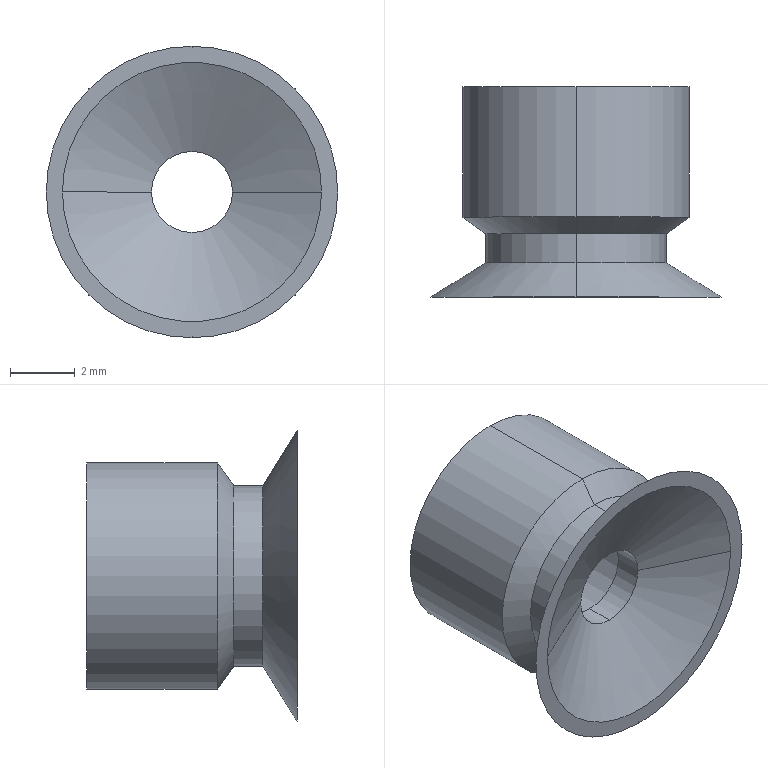Part | STEP file | PN_0033 | 1 solid | 18 faces | box 9 x 6.5 x 9 mm | volume 149.71 mm3 | cylinder 8 | cone 8 | plane 2 | commonest cylinder face diameters 2.5 x2 4.028 x2 5.56 x2 7 x2
STEP:
#1=CARTESIAN_POINT('',(0.,0.,0.));
#2=DIRECTION('',(0.,0.,1.));
#3=DIRECTION('',(1.,0.,0.));
#4=AXIS2_PLACEMENT_3D('',#1,#2,#3);
#5=CARTESIAN_POINT('',(0.,0.,-3.5));
#6=VERTEX_POINT('',#5);
#7=CARTESIAN_POINT('',(0.,0.,3.5));
#8=VERTEX_POINT('',#7);
#9=CARTESIAN_POINT('',(0.,0.,0.));
#10=DIRECTION('',(0.,-1.,0.));
#11=DIRECTION('',(0.,0.,-1.));
#12=AXIS2_PLACEMENT_3D('',#9,#10,#11);
#13=CIRCLE('',#12,3.5);
#14=CARTESIAN_POINT('',(0.,43.5,0.));
#15=DIRECTION('',(0.,-1.,0.));
#16=DIRECTION('',(0.,0.,-1.));
#17=AXIS2_PLACEMENT_3D('',#14,#15,#16);
#18=CYLINDRICAL_SURFACE('',#17,3.5);
#19=CARTESIAN_POINT('',(0.,43.5));
#20=DIRECTION('',(1.,0.));
#21=VECTOR('',#20,1.);
#22=LINE('',#19,#21);
#23=(GEOMETRIC_REPRESENTATION_CONTEXT(2)PARAMETRIC_REPRESENTATION_CONTEXT()REPRESENTATION_CONTEXT('',''));
#24=DEFINITIONAL_REPRESENTATION('',(#22),#23);
#25=PCURVE('',#18,#24);
#26=CARTESIAN_POINT('',(0.,0.,2.014));
#27=DIRECTION('',(0.,1.,0.));
#28=DIRECTION('',(0.,0.,1.));
#29=AXIS2_PLACEMENT_3D('',#26,#27,#28);
#30=PLANE('',#29);
#31=CARTESIAN_POINT('',(-5.514,0.));
#32=CARTESIAN_POINT('',(-5.514,6.062));
#33=CARTESIAN_POINT('',(-0.264,3.031));
#34=CARTESIAN_POINT('',(4.986,0.));
#35=CARTESIAN_POINT('',(-0.264,-3.031));
#36=CARTESIAN_POINT('',(-5.514,-6.062));
#37=CARTESIAN_POINT('',(-5.514,0.));
#38=(BOUNDED_CURVE()B_SPLINE_CURVE(2,(#31,#32,#33,#34,#35,#36,#37),.UNSPECIFIED.,.T.,.F.)B_SPLINE_CURVE_WITH_KNOTS((1,2,2,2,2,1),(-2.094,0.,2.094,4.189,6.283,8.378),.UNSPECIFIED.)CURVE()GEOMETRIC_REPRESENTATION_ITEM()RATIONAL_B_SPLINE_CURVE((1.,0.5,1.,0.5,1.,0.5,1.))REPRESENTATION_ITEM(''));
#39=(GEOMETRIC_REPRESENTATION_CONTEXT(2)PARAMETRIC_REPRESENTATION_CONTEXT()REPRESENTATION_CONTEXT('',''));
#40=DEFINITIONAL_REPRESENTATION('',(#38),#39);
#41=PCURVE('',#30,#40);
#42=SURFACE_CURVE('',#13,(#25,#41),.PCURVE_S1.);
#43=EDGE_CURVE('',#6,#8,#42,.T.);
#44=ORIENTED_EDGE('',*,*,#43,.T.);
#45=CARTESIAN_POINT('',(0.,-4.027,3.5));
#46=VERTEX_POINT('',#45);
#47=CARTESIAN_POINT('',(0.,43.5,3.5));
#48=DIRECTION('',(0.,-1.,0.));
#49=VECTOR('',#48,1.);
#50=LINE('',#47,#49);
#51=CARTESIAN_POINT('',(3.142,0.));
#52=DIRECTION('',(0.,1.));
#53=VECTOR('',#52,1.);
#54=LINE('',#51,#53);
#55=(GEOMETRIC_REPRESENTATION_CONTEXT(2)PARAMETRIC_REPRESENTATION_CONTEXT()REPRESENTATION_CONTEXT('',''));
#56=DEFINITIONAL_REPRESENTATION('',(#54),#55);
#57=PCURVE('',#18,#56);
#58=CARTESIAN_POINT('',(0.,43.5,0.));
#59=DIRECTION('',(0.,-1.,0.));
#60=DIRECTION('',(0.,0.,-1.));
#61=AXIS2_PLACEMENT_3D('',#58,#59,#60);
#62=CYLINDRICAL_SURFACE('',#61,3.5);
#63=CARTESIAN_POINT('',(3.142,0.));
#64=DIRECTION('',(0.,1.));
#65=VECTOR('',#64,1.);
#66=LINE('',#63,#65);
#67=(GEOMETRIC_REPRESENTATION_CONTEXT(2)PARAMETRIC_REPRESENTATION_CONTEXT()REPRESENTATION_CONTEXT('',''));
#68=DEFINITIONAL_REPRESENTATION('',(#66),#67);
#69=PCURVE('',#62,#68);
#70=SURFACE_CURVE('',#50,(#57,#69),.PCURVE_S1.);
#71=EDGE_CURVE('',#8,#46,#70,.T.);
#72=ORIENTED_EDGE('',*,*,#71,.T.);
#73=CARTESIAN_POINT('',(0.,-4.027,-3.5));
#74=VERTEX_POINT('',#73);
#75=CARTESIAN_POINT('',(0.,-4.027,0.));
#76=DIRECTION('',(0.,1.,0.));
#77=DIRECTION('',(0.,0.,-1.));
#78=AXIS2_PLACEMENT_3D('',#75,#76,#77);
#79=CIRCLE('',#78,3.5);
#80=CARTESIAN_POINT('',(6.283,47.527));
#81=DIRECTION('',(-1.,0.));
#82=VECTOR('',#81,1.);
#83=LINE('',#80,#82);
#84=(GEOMETRIC_REPRESENTATION_CONTEXT(2)PARAMETRIC_REPRESENTATION_CONTEXT()REPRESENTATION_CONTEXT('',''));
#85=DEFINITIONAL_REPRESENTATION('',(#83),#84);
#86=PCURVE('',#18,#85);
#87=CARTESIAN_POINT('',(0.,-4.027,0.));
#88=DIRECTION('',(0.,1.,0.));
#89=DIRECTION('',(0.,0.,1.));
#90=AXIS2_PLACEMENT_3D('',#87,#88,#89);
#91=CONICAL_SURFACE('',#90,3.5,0.9499);
#92=CARTESIAN_POINT('',(-3.142,0.));
#93=DIRECTION('',(1.,0.));
#94=VECTOR('',#93,1.);
#95=LINE('',#92,#94);
#96=(GEOMETRIC_REPRESENTATION_CONTEXT(2)PARAMETRIC_REPRESENTATION_CONTEXT()REPRESENTATION_CONTEXT('',''));
#97=DEFINITIONAL_REPRESENTATION('',(#95),#96);
#98=PCURVE('',#91,#97);
#99=SURFACE_CURVE('',#79,(#86,#98),.PCURVE_S1.);
#100=EDGE_CURVE('',#46,#74,#99,.T.);
#101=ORIENTED_EDGE('',*,*,#100,.T.);
#102=CARTESIAN_POINT('',(0.,43.5,-3.5));
#103=DIRECTION('',(0.,-1.,0.));
#104=VECTOR('',#103,1.);
#105=LINE('',#102,#104);
#106=CARTESIAN_POINT('',(0.,0.));
#107=DIRECTION('',(0.,1.));
#108=VECTOR('',#107,1.);
#109=LINE('',#106,#108);
#110=(GEOMETRIC_REPRESENTATION_CONTEXT(2)PARAMETRIC_REPRESENTATION_CONTEXT()REPRESENTATION_CONTEXT('',''));
#111=DEFINITIONAL_REPRESENTATION('',(#109),#110);
#112=PCURVE('',#18,#111);
#113=CARTESIAN_POINT('',(6.283,0.));
#114=DIRECTION('',(0.,1.));
#115=VECTOR('',#114,1.);
#116=LINE('',#113,#115);
#117=(GEOMETRIC_REPRESENTATION_CONTEXT(2)PARAMETRIC_REPRESENTATION_CONTEXT()REPRESENTATION_CONTEXT('',''));
#118=DEFINITIONAL_REPRESENTATION('',(#116),#117);
#119=PCURVE('',#62,#118);
#120=SURFACE_CURVE('',#105,(#112,#119),.PCURVE_S1.);
#121=EDGE_CURVE('',#6,#74,#120,.T.);
#122=ORIENTED_EDGE('',*,*,#121,.F.);
#123=EDGE_LOOP('',(#44,#72,#101,#122));
#124=FACE_BOUND('',#123,.T.);
#125=ADVANCED_FACE('',(#124),#18,.T.);
#126=CARTESIAN_POINT('',(0.,-4.542,2.78));
#127=VERTEX_POINT('',#126);
#128=CARTESIAN_POINT('',(0.,-4.542,-2.78));
#129=VERTEX_POINT('',#128);
#130=CARTESIAN_POINT('',(0.,-4.542,0.));
#131=DIRECTION('',(0.,1.,0.));
#132=DIRECTION('',(0.,0.,1.));
#133=AXIS2_PLACEMENT_3D('',#130,#131,#132);
#134=CIRCLE('',#133,2.78);
#135=CARTESIAN_POINT('',(0.,-0.515));
#136=DIRECTION('',(1.,0.));
#137=VECTOR('',#136,1.);
#138=LINE('',#135,#137);
#139=(GEOMETRIC_REPRESENTATION_CONTEXT(2)PARAMETRIC_REPRESENTATION_CONTEXT()REPRESENTATION_CONTEXT('',''));
#140=DEFINITIONAL_REPRESENTATION('',(#138),#139);
#141=PCURVE('',#91,#140);
#142=CARTESIAN_POINT('',(0.,43.5,0.));
#143=DIRECTION('',(0.,-1.,0.));
#144=DIRECTION('',(0.,0.,-1.));
#145=AXIS2_PLACEMENT_3D('',#142,#143,#144);
#146=CYLINDRICAL_SURFACE('',#145,2.78);
#147=CARTESIAN_POINT('',(3.142,48.042));
#148=DIRECTION('',(-1.,0.));
#149=VECTOR('',#148,1.);
#150=LINE('',#147,#149);
#151=(GEOMETRIC_REPRESENTATION_CONTEXT(2)PARAMETRIC_REPRESENTATION_CONTEXT()REPRESENTATION_CONTEXT('',''));
#152=DEFINITIONAL_REPRESENTATION('',(#150),#151);
#153=PCURVE('',#146,#152);
#154=SURFACE_CURVE('',#134,(#141,#153),.PCURVE_S1.);
#155=EDGE_CURVE('',#127,#129,#154,.T.);
#156=ORIENTED_EDGE('',*,*,#155,.T.);
#157=CARTESIAN_POINT('',(0.,-4.027,-3.5));
#158=DIRECTION('',(0.,0.5818,-0.8134));
#159=VECTOR('',#158,1.);
#160=LINE('',#157,#159);
#161=CARTESIAN_POINT('',(3.142,0.));
#162=DIRECTION('',(0.,1.));
#163=VECTOR('',#162,1.);
#164=LINE('',#161,#163);
#165=(GEOMETRIC_REPRESENTATION_CONTEXT(2)PARAMETRIC_REPRESENTATION_CONTEXT()REPRESENTATION_CONTEXT('',''));
#166=DEFINITIONAL_REPRESENTATION('',(#164),#165);
#167=PCURVE('',#91,#166);
#168=CARTESIAN_POINT('',(0.,-4.027,0.));
#169=DIRECTION('',(0.,1.,0.));
#170=DIRECTION('',(0.,0.,1.));
#171=AXIS2_PLACEMENT_3D('',#168,#169,#170);
#172=CONICAL_SURFACE('',#171,3.5,0.9499);
#173=CARTESIAN_POINT('',(3.142,0.));
#174=DIRECTION('',(0.,1.));
#175=VECTOR('',#174,1.);
#176=LINE('',#173,#175);
#177=(GEOMETRIC_REPRESENTATION_CONTEXT(2)PARAMETRIC_REPRESENTATION_CONTEXT()REPRESENTATION_CONTEXT('',''));
#178=DEFINITIONAL_REPRESENTATION('',(#176),#177);
#179=PCURVE('',#172,#178);
#180=SURFACE_CURVE('',#160,(#167,#179),.PCURVE_S1.);
#181=EDGE_CURVE('',#129,#74,#180,.T.);
#182=ORIENTED_EDGE('',*,*,#181,.T.);
#183=ORIENTED_EDGE('',*,*,#100,.F.);
#184=CARTESIAN_POINT('',(0.,-4.027,3.5));
#185=DIRECTION('',(0.,0.5818,0.8134));
#186=VECTOR('',#185,1.);
#187=LINE('',#184,#186);
#188=CARTESIAN_POINT('',(0.,0.));
#189=DIRECTION('',(0.,1.));
#190=VECTOR('',#189,1.);
#191=LINE('',#188,#190);
#192=(GEOMETRIC_REPRESENTATION_CONTEXT(2)PARAMETRIC_REPRESENTATION_CONTEXT()REPRESENTATION_CONTEXT('',''));
#193=DEFINITIONAL_REPRESENTATION('',(#191),#192);
#194=PCURVE('',#91,#193);
#195=CARTESIAN_POINT('',(6.283,0.));
#196=DIRECTION('',(0.,1.));
#197=VECTOR('',#196,1.);
#198=LINE('',#195,#197);
#199=(GEOMETRIC_REPRESENTATION_CONTEXT(2)PARAMETRIC_REPRESENTATION_CONTEXT()REPRESENTATION_CONTEXT('',''));
#200=DEFINITIONAL_REPRESENTATION('',(#198),#199);
#201=PCURVE('',#172,#200);
#202=SURFACE_CURVE('',#187,(#194,#201),.PCURVE_S1.);
#203=EDGE_CURVE('',#127,#46,#202,.T.);
#204=ORIENTED_EDGE('',*,*,#203,.F.);
#205=EDGE_LOOP('',(#156,#182,#183,#204));
#206=FACE_BOUND('',#205,.T.);
#207=ADVANCED_FACE('',(#206),#91,.T.);
#208=CARTESIAN_POINT('',(0.,0.,-2.014));
#209=VERTEX_POINT('',#208);
#210=CARTESIAN_POINT('',(0.,-3.84,-2.014));
#211=VERTEX_POINT('',#210);
#212=CARTESIAN_POINT('',(0.,43.5,-2.014));
#213=DIRECTION('',(0.,-1.,0.));
#214=VECTOR('',#213,1.);
#215=LINE('',#212,#214);
#216=CARTESIAN_POINT('',(0.,43.5,0.));
#217=DIRECTION('',(0.,-1.,0.));
#218=DIRECTION('',(0.,0.,-1.));
#219=AXIS2_PLACEMENT_3D('',#216,#217,#218);
#220=CYLINDRICAL_SURFACE('',#219,2.014);
#221=CARTESIAN_POINT('',(6.283,0.));
#222=DIRECTION('',(0.,1.));
#223=VECTOR('',#222,1.);
#224=LINE('',#221,#223);
#225=(GEOMETRIC_REPRESENTATION_CONTEXT(2)PARAMETRIC_REPRESENTATION_CONTEXT()REPRESENTATION_CONTEXT('',''));
#226=DEFINITIONAL_REPRESENTATION('',(#224),#225);
#227=PCURVE('',#220,#226);
#228=CARTESIAN_POINT('',(0.,43.5,0.));
#229=DIRECTION('',(0.,-1.,0.));
#230=DIRECTION('',(0.,0.,-1.));
#231=AXIS2_PLACEMENT_3D('',#228,#229,#230);
#232=CYLINDRICAL_SURFACE('',#231,2.014);
#233=CARTESIAN_POINT('',(0.,0.));
#234=DIRECTION('',(0.,1.));
#235=VECTOR('',#234,1.);
#236=LINE('',#233,#235);
#237=(GEOMETRIC_REPRESENTATION_CONTEXT(2)PARAMETRIC_REPRESENTATION_CONTEXT()REPRESENTATION_CONTEXT('',''));
#238=DEFINITIONAL_REPRESENTATION('',(#236),#237);
#239=PCURVE('',#232,#238);
#240=SURFACE_CURVE('',#215,(#227,#239),.PCURVE_S1.);
#241=EDGE_CURVE('',#209,#211,#240,.T.);
#242=ORIENTED_EDGE('',*,*,#241,.T.);
#243=CARTESIAN_POINT('',(-2.014,-3.84,0.));
#244=VERTEX_POINT('',#243);
#245=CARTESIAN_POINT('',(0.,-3.84,0.));
#246=DIRECTION('',(0.,1.,0.));
#247=DIRECTION('',(0.,0.,-1.));
#248=AXIS2_PLACEMENT_3D('',#245,#246,#247);
#249=CIRCLE('',#248,2.014);
#250=CARTESIAN_POINT('',(6.283,47.34));
#251=DIRECTION('',(-1.,0.));
#252=VECTOR('',#251,1.);
#253=LINE('',#250,#252);
#254=(GEOMETRIC_REPRESENTATION_CONTEXT(2)PARAMETRIC_REPRESENTATION_CONTEXT()REPRESENTATION_CONTEXT('',''));
#255=DEFINITIONAL_REPRESENTATION('',(#253),#254);
#256=PCURVE('',#220,#255);
#257=CARTESIAN_POINT('',(0.,-3.84,0.));
#258=DIRECTION('',(0.,1.,0.));
#259=DIRECTION('',(-1.,0.,0.));
#260=AXIS2_PLACEMENT_3D('',#257,#258,#259);
#261=CONICAL_SURFACE('',#260,2.014,0.9822);
#262=CARTESIAN_POINT('',(4.712,0.));
#263=DIRECTION('',(1.,0.));
#264=VECTOR('',#263,1.);
#265=LINE('',#262,#264);
#266=(GEOMETRIC_REPRESENTATION_CONTEXT(2)PARAMETRIC_REPRESENTATION_CONTEXT()REPRESENTATION_CONTEXT('',''));
#267=DEFINITIONAL_REPRESENTATION('',(#265),#266);
#268=PCURVE('',#261,#267);
#269=SURFACE_CURVE('',#249,(#256,#268),.PCURVE_S1.);
#270=EDGE_CURVE('',#211,#244,#269,.T.);
#271=ORIENTED_EDGE('',*,*,#270,.T.);
#272=CARTESIAN_POINT('',(0.,-3.84,2.014));
#273=VERTEX_POINT('',#272);
#274=CARTESIAN_POINT('',(0.,-3.84,0.));
#275=DIRECTION('',(0.,1.,0.));
#276=DIRECTION('',(0.,0.,-1.));
#277=AXIS2_PLACEMENT_3D('',#274,#275,#276);
#278=CIRCLE('',#277,2.014);
#279=CARTESIAN_POINT('',(6.283,47.34));
#280=DIRECTION('',(-1.,0.));
#281=VECTOR('',#280,1.);
#282=LINE('',#279,#281);
#283=(GEOMETRIC_REPRESENTATION_CONTEXT(2)PARAMETRIC_REPRESENTATION_CONTEXT()REPRESENTATION_CONTEXT('',''));
#284=DEFINITIONAL_REPRESENTATION('',(#282),#283);
#285=PCURVE('',#220,#284);
#286=CARTESIAN_POINT('',(0.,-3.84,0.));
#287=DIRECTION('',(0.,1.,0.));
#288=DIRECTION('',(-1.,0.,0.));
#289=AXIS2_PLACEMENT_3D('',#286,#287,#288);
#290=CONICAL_SURFACE('',#289,2.014,0.9822);
#291=CARTESIAN_POINT('',(-1.571,0.));
#292=DIRECTION('',(1.,0.));
#293=VECTOR('',#292,1.);
#294=LINE('',#291,#293);
#295=(GEOMETRIC_REPRESENTATION_CONTEXT(2)PARAMETRIC_REPRESENTATION_CONTEXT()REPRESENTATION_CONTEXT('',''));
#296=DEFINITIONAL_REPRESENTATION('',(#294),#295);
#297=PCURVE('',#290,#296);
#298=SURFACE_CURVE('',#278,(#285,#297),.PCURVE_S1.);
#299=EDGE_CURVE('',#244,#273,#298,.T.);
#300=ORIENTED_EDGE('',*,*,#299,.T.);
#301=CARTESIAN_POINT('',(0.,0.,2.014));
#302=VERTEX_POINT('',#301);
#303=CARTESIAN_POINT('',(0.,43.5,2.014));
#304=DIRECTION('',(0.,-1.,0.));
#305=VECTOR('',#304,1.);
#306=LINE('',#303,#305);
#307=CARTESIAN_POINT('',(3.142,0.));
#308=DIRECTION('',(0.,1.));
#309=VECTOR('',#308,1.);
#310=LINE('',#307,#309);
#311=(GEOMETRIC_REPRESENTATION_CONTEXT(2)PARAMETRIC_REPRESENTATION_CONTEXT()REPRESENTATION_CONTEXT('',''));
#312=DEFINITIONAL_REPRESENTATION('',(#310),#311);
#313=PCURVE('',#220,#312);
#314=CARTESIAN_POINT('',(3.142,0.));
#315=DIRECTION('',(0.,1.));
#316=VECTOR('',#315,1.);
#317=LINE('',#314,#316);
#318=(GEOMETRIC_REPRESENTATION_CONTEXT(2)PARAMETRIC_REPRESENTATION_CONTEXT()REPRESENTATION_CONTEXT('',''));
#319=DEFINITIONAL_REPRESENTATION('',(#317),#318);
#320=PCURVE('',#232,#319);
#321=SURFACE_CURVE('',#306,(#313,#320),.PCURVE_S1.);
#322=EDGE_CURVE('',#302,#273,#321,.T.);
#323=ORIENTED_EDGE('',*,*,#322,.F.);
#324=CARTESIAN_POINT('',(0.,0.,0.));
#325=DIRECTION('',(0.,-1.,0.));
#326=DIRECTION('',(0.,0.,-1.));
#327=AXIS2_PLACEMENT_3D('',#324,#325,#326);
#328=CIRCLE('',#327,2.014);
#329=CARTESIAN_POINT('',(0.,43.5));
#330=DIRECTION('',(1.,0.));
#331=VECTOR('',#330,1.);
#332=LINE('',#329,#331);
#333=(GEOMETRIC_REPRESENTATION_CONTEXT(2)PARAMETRIC_REPRESENTATION_CONTEXT()REPRESENTATION_CONTEXT('',''));
#334=DEFINITIONAL_REPRESENTATION('',(#332),#333);
#335=PCURVE('',#220,#334);
#336=CARTESIAN_POINT('',(-4.028,0.));
#337=CARTESIAN_POINT('',(-4.028,3.488));
#338=CARTESIAN_POINT('',(-1.007,1.744));
#339=CARTESIAN_POINT('',(2.014,0.));
#340=CARTESIAN_POINT('',(-1.007,-1.744));
#341=CARTESIAN_POINT('',(-4.028,-3.488));
#342=CARTESIAN_POINT('',(-4.028,0.));
#343=(BOUNDED_CURVE()B_SPLINE_CURVE(2,(#336,#337,#338,#339,#340,#341,#342),.UNSPECIFIED.,.T.,.F.)B_SPLINE_CURVE_WITH_KNOTS((1,2,2,2,2,1),(-2.094,0.,2.094,4.189,6.283,8.378),.UNSPECIFIED.)CURVE()GEOMETRIC_REPRESENTATION_ITEM()RATIONAL_B_SPLINE_CURVE((1.,0.5,1.,0.5,1.,0.5,1.))REPRESENTATION_ITEM(''));
#344=(GEOMETRIC_REPRESENTATION_CONTEXT(2)PARAMETRIC_REPRESENTATION_CONTEXT()REPRESENTATION_CONTEXT('',''));
#345=DEFINITIONAL_REPRESENTATION('',(#343),#344);
#346=PCURVE('',#30,#345);
#347=SURFACE_CURVE('',#328,(#335,#346),.PCURVE_S1.);
#348=EDGE_CURVE('',#302,#209,#347,.T.);
#349=ORIENTED_EDGE('',*,*,#348,.T.);
#350=EDGE_LOOP('',(#242,#271,#300,#323,#349));
#351=FACE_BOUND('',#350,.F.);
#352=ADVANCED_FACE('',(#351),#220,.F.);
#353=ORIENTED_EDGE('',*,*,#155,.F.);
#354=CARTESIAN_POINT('',(0.,-5.439,2.78));
#355=VERTEX_POINT('',#354);
#356=CARTESIAN_POINT('',(0.,43.5,2.78));
#357=DIRECTION('',(0.,-1.,0.));
#358=VECTOR('',#357,1.);
#359=LINE('',#356,#358);
#360=CARTESIAN_POINT('',(3.142,0.));
#361=DIRECTION('',(0.,1.));
#362=VECTOR('',#361,1.);
#363=LINE('',#360,#362);
#364=(GEOMETRIC_REPRESENTATION_CONTEXT(2)PARAMETRIC_REPRESENTATION_CONTEXT()REPRESENTATION_CONTEXT('',''));
#365=DEFINITIONAL_REPRESENTATION('',(#363),#364);
#366=PCURVE('',#146,#365);
#367=CARTESIAN_POINT('',(0.,43.5,0.));
#368=DIRECTION('',(0.,-1.,0.));
#369=DIRECTION('',(0.,0.,-1.));
#370=AXIS2_PLACEMENT_3D('',#367,#368,#369);
#371=CYLINDRICAL_SURFACE('',#370,2.78);
#372=CARTESIAN_POINT('',(3.142,0.));
#373=DIRECTION('',(0.,1.));
#374=VECTOR('',#373,1.);
#375=LINE('',#372,#374);
#376=(GEOMETRIC_REPRESENTATION_CONTEXT(2)PARAMETRIC_REPRESENTATION_CONTEXT()REPRESENTATION_CONTEXT('',''));
#377=DEFINITIONAL_REPRESENTATION('',(#375),#376);
#378=PCURVE('',#371,#377);
#379=SURFACE_CURVE('',#359,(#366,#378),.PCURVE_S1.);
#380=EDGE_CURVE('',#127,#355,#379,.T.);
#381=ORIENTED_EDGE('',*,*,#380,.T.);
#382=CARTESIAN_POINT('',(0.,-5.439,-2.78));
#383=VERTEX_POINT('',#382);
#384=CARTESIAN_POINT('',(0.,-5.439,0.));
#385=DIRECTION('',(0.,1.,0.));
#386=DIRECTION('',(0.,0.,-1.));
#387=AXIS2_PLACEMENT_3D('',#384,#385,#386);
#388=CIRCLE('',#387,2.78);
#389=CARTESIAN_POINT('',(6.283,48.939));
#390=DIRECTION('',(-1.,0.));
#391=VECTOR('',#390,1.);
#392=LINE('',#389,#391);
#393=(GEOMETRIC_REPRESENTATION_CONTEXT(2)PARAMETRIC_REPRESENTATION_CONTEXT()REPRESENTATION_CONTEXT('',''));
#394=DEFINITIONAL_REPRESENTATION('',(#392),#393);
#395=PCURVE('',#146,#394);
#396=CARTESIAN_POINT('',(0.,-6.5,0.));
#397=DIRECTION('',(0.,-1.,0.));
#398=DIRECTION('',(0.,0.,-1.));
#399=AXIS2_PLACEMENT_3D('',#396,#397,#398);
#400=CONICAL_SURFACE('',#399,4.5,1.018);
#401=CARTESIAN_POINT('',(6.283,-1.061));
#402=DIRECTION('',(-1.,0.));
#403=VECTOR('',#402,1.);
#404=LINE('',#401,#403);
#405=(GEOMETRIC_REPRESENTATION_CONTEXT(2)PARAMETRIC_REPRESENTATION_CONTEXT()REPRESENTATION_CONTEXT('',''));
#406=DEFINITIONAL_REPRESENTATION('',(#404),#405);
#407=PCURVE('',#400,#406);
#408=SURFACE_CURVE('',#388,(#395,#407),.PCURVE_S1.);
#409=EDGE_CURVE('',#355,#383,#408,.T.);
#410=ORIENTED_EDGE('',*,*,#409,.T.);
#411=CARTESIAN_POINT('',(0.,43.5,-2.78));
#412=DIRECTION('',(0.,-1.,0.));
#413=VECTOR('',#412,1.);
#414=LINE('',#411,#413);
#415=CARTESIAN_POINT('',(0.,0.));
#416=DIRECTION('',(0.,1.));
#417=VECTOR('',#416,1.);
#418=LINE('',#415,#417);
#419=(GEOMETRIC_REPRESENTATION_CONTEXT(2)PARAMETRIC_REPRESENTATION_CONTEXT()REPRESENTATION_CONTEXT('',''));
#420=DEFINITIONAL_REPRESENTATION('',(#418),#419);
#421=PCURVE('',#146,#420);
#422=CARTESIAN_POINT('',(6.283,0.));
#423=DIRECTION('',(0.,1.));
#424=VECTOR('',#423,1.);
#425=LINE('',#422,#424);
#426=(GEOMETRIC_REPRESENTATION_CONTEXT(2)PARAMETRIC_REPRESENTATION_CONTEXT()REPRESENTATION_CONTEXT('',''));
#427=DEFINITIONAL_REPRESENTATION('',(#425),#426);
#428=PCURVE('',#371,#427);
#429=SURFACE_CURVE('',#414,(#421,#428),.PCURVE_S1.);
#430=EDGE_CURVE('',#129,#383,#429,.T.);
#431=ORIENTED_EDGE('',*,*,#430,.F.);
#432=EDGE_LOOP('',(#353,#381,#410,#431));
#433=FACE_BOUND('',#432,.T.);
#434=ADVANCED_FACE('',(#433),#146,.T.);
#435=CARTESIAN_POINT('',(0.,-4.35,-1.25));
#436=VERTEX_POINT('',#435);
#437=CARTESIAN_POINT('',(-1.25,-4.35,0.));
#438=VERTEX_POINT('',#437);
#439=CARTESIAN_POINT('',(0.,-4.35,0.));
#440=DIRECTION('',(0.,1.,0.));
#441=DIRECTION('',(0.,0.,1.));
#442=AXIS2_PLACEMENT_3D('',#439,#440,#441);
#443=CIRCLE('',#442,1.25);
#444=CARTESIAN_POINT('',(1.571,-0.51));
#445=DIRECTION('',(1.,0.));
#446=VECTOR('',#445,1.);
#447=LINE('',#444,#446);
#448=(GEOMETRIC_REPRESENTATION_CONTEXT(2)PARAMETRIC_REPRESENTATION_CONTEXT()REPRESENTATION_CONTEXT('',''));
#449=DEFINITIONAL_REPRESENTATION('',(#447),#448);
#450=PCURVE('',#261,#449);
#451=CARTESIAN_POINT('',(0.,43.5,0.));
#452=DIRECTION('',(0.,-1.,0.));
#453=DIRECTION('',(0.,0.,-1.));
#454=AXIS2_PLACEMENT_3D('',#451,#452,#453);
#455=CYLINDRICAL_SURFACE('',#454,1.25);
#456=CARTESIAN_POINT('',(9.425,47.85));
#457=DIRECTION('',(-1.,0.));
#458=VECTOR('',#457,1.);
#459=LINE('',#456,#458);
#460=(GEOMETRIC_REPRESENTATION_CONTEXT(2)PARAMETRIC_REPRESENTATION_CONTEXT()REPRESENTATION_CONTEXT('',''));
#461=DEFINITIONAL_REPRESENTATION('',(#459),#460);
#462=PCURVE('',#455,#461);
#463=SURFACE_CURVE('',#443,(#450,#462),.PCURVE_S1.);
#464=EDGE_CURVE('',#436,#438,#463,.T.);
#465=ORIENTED_EDGE('',*,*,#464,.T.);
#466=CARTESIAN_POINT('',(-2.014,-3.84,0.));
#467=DIRECTION('',(-0.8317,0.5552,0.));
#468=VECTOR('',#467,1.);
#469=LINE('',#466,#468);
#470=CARTESIAN_POINT('',(6.283,0.));
#471=DIRECTION('',(0.,1.));
#472=VECTOR('',#471,1.);
#473=LINE('',#470,#472);
#474=(GEOMETRIC_REPRESENTATION_CONTEXT(2)PARAMETRIC_REPRESENTATION_CONTEXT()REPRESENTATION_CONTEXT('',''));
#475=DEFINITIONAL_REPRESENTATION('',(#473),#474);
#476=PCURVE('',#261,#475);
#477=CARTESIAN_POINT('',(0.,0.));
#478=DIRECTION('',(0.,1.));
#479=VECTOR('',#478,1.);
#480=LINE('',#477,#479);
#481=(GEOMETRIC_REPRESENTATION_CONTEXT(2)PARAMETRIC_REPRESENTATION_CONTEXT()REPRESENTATION_CONTEXT('',''));
#482=DEFINITIONAL_REPRESENTATION('',(#480),#481);
#483=PCURVE('',#290,#482);
#484=SURFACE_CURVE('',#469,(#476,#483),.PCURVE_S1.);
#485=EDGE_CURVE('',#438,#244,#484,.T.);
#486=ORIENTED_EDGE('',*,*,#485,.T.);
#487=ORIENTED_EDGE('',*,*,#270,.F.);
#488=CARTESIAN_POINT('',(2.014,-3.84,0.));
#489=VERTEX_POINT('',#488);
#490=CARTESIAN_POINT('',(0.,-3.84,0.));
#491=DIRECTION('',(0.,1.,0.));
#492=DIRECTION('',(0.,0.,-1.));
#493=AXIS2_PLACEMENT_3D('',#490,#491,#492);
#494=CIRCLE('',#493,2.014);
#495=CARTESIAN_POINT('',(-1.571,0.));
#496=DIRECTION('',(1.,0.));
#497=VECTOR('',#496,1.);
#498=LINE('',#495,#497);
#499=(GEOMETRIC_REPRESENTATION_CONTEXT(2)PARAMETRIC_REPRESENTATION_CONTEXT()REPRESENTATION_CONTEXT('',''));
#500=DEFINITIONAL_REPRESENTATION('',(#498),#499);
#501=PCURVE('',#261,#500);
#502=CARTESIAN_POINT('',(6.283,47.34));
#503=DIRECTION('',(-1.,0.));
#504=VECTOR('',#503,1.);
#505=LINE('',#502,#504);
#506=(GEOMETRIC_REPRESENTATION_CONTEXT(2)PARAMETRIC_REPRESENTATION_CONTEXT()REPRESENTATION_CONTEXT('',''));
#507=DEFINITIONAL_REPRESENTATION('',(#505),#506);
#508=PCURVE('',#232,#507);
#509=SURFACE_CURVE('',#494,(#501,#508),.PCURVE_S1.);
#510=EDGE_CURVE('',#489,#211,#509,.T.);
#511=ORIENTED_EDGE('',*,*,#510,.F.);
#512=CARTESIAN_POINT('',(1.25,-4.35,0.));
#513=VERTEX_POINT('',#512);
#514=CARTESIAN_POINT('',(2.014,-3.84,0.));
#515=DIRECTION('',(0.8317,0.5552,0.));
#516=VECTOR('',#515,1.);
#517=LINE('',#514,#516);
#518=CARTESIAN_POINT('',(3.142,0.));
#519=DIRECTION('',(0.,1.));
#520=VECTOR('',#519,1.);
#521=LINE('',#518,#520);
#522=(GEOMETRIC_REPRESENTATION_CONTEXT(2)PARAMETRIC_REPRESENTATION_CONTEXT()REPRESENTATION_CONTEXT('',''));
#523=DEFINITIONAL_REPRESENTATION('',(#521),#522);
#524=PCURVE('',#261,#523);
#525=CARTESIAN_POINT('',(3.142,0.));
#526=DIRECTION('',(0.,1.));
#527=VECTOR('',#526,1.);
#528=LINE('',#525,#527);
#529=(GEOMETRIC_REPRESENTATION_CONTEXT(2)PARAMETRIC_REPRESENTATION_CONTEXT()REPRESENTATION_CONTEXT('',''));
#530=DEFINITIONAL_REPRESENTATION('',(#528),#529);
#531=PCURVE('',#290,#530);
#532=SURFACE_CURVE('',#517,(#524,#531),.PCURVE_S1.);
#533=EDGE_CURVE('',#513,#489,#532,.T.);
#534=ORIENTED_EDGE('',*,*,#533,.F.);
#535=CARTESIAN_POINT('',(0.,-4.35,0.));
#536=DIRECTION('',(0.,1.,0.));
#537=DIRECTION('',(0.,0.,1.));
#538=AXIS2_PLACEMENT_3D('',#535,#536,#537);
#539=CIRCLE('',#538,1.25);
#540=CARTESIAN_POINT('',(1.571,-0.51));
#541=DIRECTION('',(1.,0.));
#542=VECTOR('',#541,1.);
#543=LINE('',#540,#542);
#544=(GEOMETRIC_REPRESENTATION_CONTEXT(2)PARAMETRIC_REPRESENTATION_CONTEXT()REPRESENTATION_CONTEXT('',''));
#545=DEFINITIONAL_REPRESENTATION('',(#543),#544);
#546=PCURVE('',#261,#545);
#547=CARTESIAN_POINT('',(0.,43.5,0.));
#548=DIRECTION('',(0.,-1.,0.));
#549=DIRECTION('',(0.,0.,-1.));
#550=AXIS2_PLACEMENT_3D('',#547,#548,#549);
#551=CYLINDRICAL_SURFACE('',#550,1.25);
#552=CARTESIAN_POINT('',(3.142,47.85));
#553=DIRECTION('',(-1.,0.));
#554=VECTOR('',#553,1.);
#555=LINE('',#552,#554);
#556=(GEOMETRIC_REPRESENTATION_CONTEXT(2)PARAMETRIC_REPRESENTATION_CONTEXT()REPRESENTATION_CONTEXT('',''));
#557=DEFINITIONAL_REPRESENTATION('',(#555),#556);
#558=PCURVE('',#551,#557);
#559=SURFACE_CURVE('',#539,(#546,#558),.PCURVE_S1.);
#560=EDGE_CURVE('',#513,#436,#559,.T.);
#561=ORIENTED_EDGE('',*,*,#560,.T.);
#562=EDGE_LOOP('',(#465,#486,#487,#511,#534,#561));
#563=FACE_BOUND('',#562,.F.);
#564=ADVANCED_FACE('',(#563),#261,.F.);
#565=ORIENTED_EDGE('',*,*,#409,.F.);
#566=CARTESIAN_POINT('',(0.,-6.5,4.5));
#567=VERTEX_POINT('',#566);
#568=CARTESIAN_POINT('',(0.,-6.5,4.5));
#569=DIRECTION('',(0.,-0.525,0.8511));
#570=VECTOR('',#569,1.);
#571=LINE('',#568,#570);
#572=CARTESIAN_POINT('',(3.142,0.));
#573=DIRECTION('',(0.,1.));
#574=VECTOR('',#573,1.);
#575=LINE('',#572,#574);
#576=(GEOMETRIC_REPRESENTATION_CONTEXT(2)PARAMETRIC_REPRESENTATION_CONTEXT()REPRESENTATION_CONTEXT('',''));
#577=DEFINITIONAL_REPRESENTATION('',(#575),#576);
#578=PCURVE('',#400,#577);
#579=CARTESIAN_POINT('',(0.,-6.5,0.));
#580=DIRECTION('',(0.,-1.,0.));
#581=DIRECTION('',(0.,0.,-1.));
#582=AXIS2_PLACEMENT_3D('',#579,#580,#581);
#583=CONICAL_SURFACE('',#582,4.5,1.018);
#584=CARTESIAN_POINT('',(3.142,0.));
#585=DIRECTION('',(0.,1.));
#586=VECTOR('',#585,1.);
#587=LINE('',#584,#586);
#588=(GEOMETRIC_REPRESENTATION_CONTEXT(2)PARAMETRIC_REPRESENTATION_CONTEXT()REPRESENTATION_CONTEXT('',''));
#589=DEFINITIONAL_REPRESENTATION('',(#587),#588);
#590=PCURVE('',#583,#589);
#591=SURFACE_CURVE('',#571,(#578,#590),.PCURVE_S1.);
#592=EDGE_CURVE('',#355,#567,#591,.T.);
#593=ORIENTED_EDGE('',*,*,#592,.T.);
#594=CARTESIAN_POINT('',(0.,-6.5,-4.5));
#595=VERTEX_POINT('',#594);
#596=CARTESIAN_POINT('',(0.,-6.5,0.));
#597=DIRECTION('',(0.,1.,0.));
#598=DIRECTION('',(0.,0.,-1.));
#599=AXIS2_PLACEMENT_3D('',#596,#597,#598);
#600=CIRCLE('',#599,4.5);
#601=CARTESIAN_POINT('',(6.283,0.));
#602=DIRECTION('',(-1.,0.));
#603=VECTOR('',#602,1.);
#604=LINE('',#601,#603);
#605=(GEOMETRIC_REPRESENTATION_CONTEXT(2)PARAMETRIC_REPRESENTATION_CONTEXT()REPRESENTATION_CONTEXT('',''));
#606=DEFINITIONAL_REPRESENTATION('',(#604),#605);
#607=PCURVE('',#400,#606);
#608=CARTESIAN_POINT('',(0.,-6.5,4.5));
#609=DIRECTION('',(0.,-1.,0.));
#610=DIRECTION('',(0.,0.,-1.));
#611=AXIS2_PLACEMENT_3D('',#608,#609,#610);
#612=PLANE('',#611);
#613=CARTESIAN_POINT('',(9.,0.));
#614=CARTESIAN_POINT('',(9.,-7.794));
#615=CARTESIAN_POINT('',(2.25,-3.897));
#616=CARTESIAN_POINT('',(-4.5,0.));
#617=CARTESIAN_POINT('',(2.25,3.897));
#618=CARTESIAN_POINT('',(9.,7.794));
#619=CARTESIAN_POINT('',(9.,0.));
#620=(BOUNDED_CURVE()B_SPLINE_CURVE(2,(#613,#614,#615,#616,#617,#618,#619),.UNSPECIFIED.,.T.,.F.)B_SPLINE_CURVE_WITH_KNOTS((1,2,2,2,2,1),(-2.094,0.,2.094,4.189,6.283,8.378),.UNSPECIFIED.)CURVE()GEOMETRIC_REPRESENTATION_ITEM()RATIONAL_B_SPLINE_CURVE((1.,0.5,1.,0.5,1.,0.5,1.))REPRESENTATION_ITEM(''));
#621=(GEOMETRIC_REPRESENTATION_CONTEXT(2)PARAMETRIC_REPRESENTATION_CONTEXT()REPRESENTATION_CONTEXT('',''));
#622=DEFINITIONAL_REPRESENTATION('',(#620),#621);
#623=PCURVE('',#612,#622);
#624=SURFACE_CURVE('',#600,(#607,#623),.PCURVE_S1.);
#625=EDGE_CURVE('',#567,#595,#624,.T.);
#626=ORIENTED_EDGE('',*,*,#625,.T.);
#627=CARTESIAN_POINT('',(0.,-6.5,-4.5));
#628=DIRECTION('',(0.,-0.525,-0.8511));
#629=VECTOR('',#628,1.);
#630=LINE('',#627,#629);
#631=CARTESIAN_POINT('',(0.,0.));
#632=DIRECTION('',(0.,1.));
#633=VECTOR('',#632,1.);
#634=LINE('',#631,#633);
#635=(GEOMETRIC_REPRESENTATION_CONTEXT(2)PARAMETRIC_REPRESENTATION_CONTEXT()REPRESENTATION_CONTEXT('',''));
#636=DEFINITIONAL_REPRESENTATION('',(#634),#635);
#637=PCURVE('',#400,#636);
#638=CARTESIAN_POINT('',(6.283,0.));
#639=DIRECTION('',(0.,1.));
#640=VECTOR('',#639,1.);
#641=LINE('',#638,#640);
#642=(GEOMETRIC_REPRESENTATION_CONTEXT(2)PARAMETRIC_REPRESENTATION_CONTEXT()REPRESENTATION_CONTEXT('',''));
#643=DEFINITIONAL_REPRESENTATION('',(#641),#642);
#644=PCURVE('',#583,#643);
#645=SURFACE_CURVE('',#630,(#637,#644),.PCURVE_S1.);
#646=EDGE_CURVE('',#383,#595,#645,.T.);
#647=ORIENTED_EDGE('',*,*,#646,.F.);
#648=EDGE_LOOP('',(#565,#593,#626,#647));
#649=FACE_BOUND('',#648,.T.);
#650=ADVANCED_FACE('',(#649),#400,.T.);
#651=CARTESIAN_POINT('',(0.,-5.206,-1.25));
#652=VERTEX_POINT('',#651);
#653=CARTESIAN_POINT('',(0.,43.5,-1.25));
#654=DIRECTION('',(0.,-1.,0.));
#655=VECTOR('',#654,1.);
#656=LINE('',#653,#655);
#657=CARTESIAN_POINT('',(6.283,0.));
#658=DIRECTION('',(0.,1.));
#659=VECTOR('',#658,1.);
#660=LINE('',#657,#659);
#661=(GEOMETRIC_REPRESENTATION_CONTEXT(2)PARAMETRIC_REPRESENTATION_CONTEXT()REPRESENTATION_CONTEXT('',''));
#662=DEFINITIONAL_REPRESENTATION('',(#660),#661);
#663=PCURVE('',#455,#662);
#664=CARTESIAN_POINT('',(0.,0.));
#665=DIRECTION('',(0.,1.));
#666=VECTOR('',#665,1.);
#667=LINE('',#664,#666);
#668=(GEOMETRIC_REPRESENTATION_CONTEXT(2)PARAMETRIC_REPRESENTATION_CONTEXT()REPRESENTATION_CONTEXT('',''));
#669=DEFINITIONAL_REPRESENTATION('',(#667),#668);
#670=PCURVE('',#551,#669);
#671=SURFACE_CURVE('',#656,(#663,#670),.PCURVE_S1.);
#672=EDGE_CURVE('',#436,#652,#671,.T.);
#673=ORIENTED_EDGE('',*,*,#672,.T.);
#674=CARTESIAN_POINT('',(-1.25,-5.206,0.));
#675=VERTEX_POINT('',#674);
#676=CARTESIAN_POINT('',(0.,-5.206,0.));
#677=DIRECTION('',(0.,1.,0.));
#678=DIRECTION('',(0.,0.,-1.));
#679=AXIS2_PLACEMENT_3D('',#676,#677,#678);
#680=CIRCLE('',#679,1.25);
#681=CARTESIAN_POINT('',(6.283,48.706));
#682=DIRECTION('',(-1.,0.));
#683=VECTOR('',#682,1.);
#684=LINE('',#681,#683);
#685=(GEOMETRIC_REPRESENTATION_CONTEXT(2)PARAMETRIC_REPRESENTATION_CONTEXT()REPRESENTATION_CONTEXT('',''));
#686=DEFINITIONAL_REPRESENTATION('',(#684),#685);
#687=PCURVE('',#455,#686);
#688=CARTESIAN_POINT('',(0.,-6.5,0.));
#689=DIRECTION('',(0.,-1.,0.));
#690=DIRECTION('',(1.,0.,0.));
#691=AXIS2_PLACEMENT_3D('',#688,#689,#690);
#692=CONICAL_SURFACE('',#691,4.,1.131);
#693=CARTESIAN_POINT('',(4.712,-1.294));
#694=DIRECTION('',(-1.,0.));
#695=VECTOR('',#694,1.);
#696=LINE('',#693,#695);
#697=(GEOMETRIC_REPRESENTATION_CONTEXT(2)PARAMETRIC_REPRESENTATION_CONTEXT()REPRESENTATION_CONTEXT('',''));
#698=DEFINITIONAL_REPRESENTATION('',(#696),#697);
#699=PCURVE('',#692,#698);
#700=SURFACE_CURVE('',#680,(#687,#699),.PCURVE_S1.);
#701=EDGE_CURVE('',#652,#675,#700,.T.);
#702=ORIENTED_EDGE('',*,*,#701,.T.);
#703=CARTESIAN_POINT('',(0.,-5.206,1.25));
#704=VERTEX_POINT('',#703);
#705=CARTESIAN_POINT('',(0.,-5.206,0.));
#706=DIRECTION('',(0.,1.,0.));
#707=DIRECTION('',(0.,0.,-1.));
#708=AXIS2_PLACEMENT_3D('',#705,#706,#707);
#709=CIRCLE('',#708,1.25);
#710=CARTESIAN_POINT('',(6.283,48.706));
#711=DIRECTION('',(-1.,0.));
#712=VECTOR('',#711,1.);
#713=LINE('',#710,#712);
#714=(GEOMETRIC_REPRESENTATION_CONTEXT(2)PARAMETRIC_REPRESENTATION_CONTEXT()REPRESENTATION_CONTEXT('',''));
#715=DEFINITIONAL_REPRESENTATION('',(#713),#714);
#716=PCURVE('',#455,#715);
#717=CARTESIAN_POINT('',(0.,-6.5,0.));
#718=DIRECTION('',(0.,-1.,0.));
#719=DIRECTION('',(1.,0.,0.));
#720=AXIS2_PLACEMENT_3D('',#717,#718,#719);
#721=CONICAL_SURFACE('',#720,4.,1.131);
#722=CARTESIAN_POINT('',(4.712,-1.294));
#723=DIRECTION('',(-1.,0.));
#724=VECTOR('',#723,1.);
#725=LINE('',#722,#724);
#726=(GEOMETRIC_REPRESENTATION_CONTEXT(2)PARAMETRIC_REPRESENTATION_CONTEXT()REPRESENTATION_CONTEXT('',''));
#727=DEFINITIONAL_REPRESENTATION('',(#725),#726);
#728=PCURVE('',#721,#727);
#729=SURFACE_CURVE('',#709,(#716,#728),.PCURVE_S1.);
#730=EDGE_CURVE('',#675,#704,#729,.T.);
#731=ORIENTED_EDGE('',*,*,#730,.T.);
#732=CARTESIAN_POINT('',(0.,-4.35,1.25));
#733=VERTEX_POINT('',#732);
#734=CARTESIAN_POINT('',(0.,43.5,1.25));
#735=DIRECTION('',(0.,-1.,0.));
#736=VECTOR('',#735,1.);
#737=LINE('',#734,#736);
#738=CARTESIAN_POINT('',(3.142,0.));
#739=DIRECTION('',(0.,1.));
#740=VECTOR('',#739,1.);
#741=LINE('',#738,#740);
#742=(GEOMETRIC_REPRESENTATION_CONTEXT(2)PARAMETRIC_REPRESENTATION_CONTEXT()REPRESENTATION_CONTEXT('',''));
#743=DEFINITIONAL_REPRESENTATION('',(#741),#742);
#744=PCURVE('',#455,#743);
#745=CARTESIAN_POINT('',(3.142,0.));
#746=DIRECTION('',(0.,1.));
#747=VECTOR('',#746,1.);
#748=LINE('',#745,#747);
#749=(GEOMETRIC_REPRESENTATION_CONTEXT(2)PARAMETRIC_REPRESENTATION_CONTEXT()REPRESENTATION_CONTEXT('',''));
#750=DEFINITIONAL_REPRESENTATION('',(#748),#749);
#751=PCURVE('',#551,#750);
#752=SURFACE_CURVE('',#737,(#744,#751),.PCURVE_S1.);
#753=EDGE_CURVE('',#733,#704,#752,.T.);
#754=ORIENTED_EDGE('',*,*,#753,.F.);
#755=CARTESIAN_POINT('',(0.,-4.35,0.));
#756=DIRECTION('',(0.,1.,0.));
#757=DIRECTION('',(0.,0.,1.));
#758=AXIS2_PLACEMENT_3D('',#755,#756,#757);
#759=CIRCLE('',#758,1.25);
#760=CARTESIAN_POINT('',(9.425,47.85));
#761=DIRECTION('',(-1.,0.));
#762=VECTOR('',#761,1.);
#763=LINE('',#760,#762);
#764=(GEOMETRIC_REPRESENTATION_CONTEXT(2)PARAMETRIC_REPRESENTATION_CONTEXT()REPRESENTATION_CONTEXT('',''));
#765=DEFINITIONAL_REPRESENTATION('',(#763),#764);
#766=PCURVE('',#455,#765);
#767=CARTESIAN_POINT('',(-4.712,-0.51));
#768=DIRECTION('',(1.,0.));
#769=VECTOR('',#768,1.);
#770=LINE('',#767,#769);
#771=(GEOMETRIC_REPRESENTATION_CONTEXT(2)PARAMETRIC_REPRESENTATION_CONTEXT()REPRESENTATION_CONTEXT('',''));
#772=DEFINITIONAL_REPRESENTATION('',(#770),#771);
#773=PCURVE('',#290,#772);
#774=SURFACE_CURVE('',#759,(#766,#773),.PCURVE_S1.);
#775=EDGE_CURVE('',#438,#733,#774,.T.);
#776=ORIENTED_EDGE('',*,*,#775,.F.);
#777=ORIENTED_EDGE('',*,*,#464,.F.);
#778=EDGE_LOOP('',(#673,#702,#731,#754,#776,#777));
#779=FACE_BOUND('',#778,.F.);
#780=ADVANCED_FACE('',(#779),#455,.F.);
#781=CARTESIAN_POINT('',(1.25,-5.206,0.));
#782=VERTEX_POINT('',#781);
#783=CARTESIAN_POINT('',(4.,-6.5,0.));
#784=VERTEX_POINT('',#783);
#785=CARTESIAN_POINT('',(4.,-6.5,0.));
#786=DIRECTION('',(0.9048,-0.4258,0.));
#787=VECTOR('',#786,1.);
#788=LINE('',#785,#787);
#789=CARTESIAN_POINT('',(6.283,0.));
#790=DIRECTION('',(0.,1.));
#791=VECTOR('',#790,1.);
#792=LINE('',#789,#791);
#793=(GEOMETRIC_REPRESENTATION_CONTEXT(2)PARAMETRIC_REPRESENTATION_CONTEXT()REPRESENTATION_CONTEXT('',''));
#794=DEFINITIONAL_REPRESENTATION('',(#792),#793);
#795=PCURVE('',#692,#794);
#796=CARTESIAN_POINT('',(0.,0.));
#797=DIRECTION('',(0.,1.));
#798=VECTOR('',#797,1.);
#799=LINE('',#796,#798);
#800=(GEOMETRIC_REPRESENTATION_CONTEXT(2)PARAMETRIC_REPRESENTATION_CONTEXT()REPRESENTATION_CONTEXT('',''));
#801=DEFINITIONAL_REPRESENTATION('',(#799),#800);
#802=PCURVE('',#721,#801);
#803=SURFACE_CURVE('',#788,(#795,#802),.PCURVE_S1.);
#804=EDGE_CURVE('',#782,#784,#803,.T.);
#805=ORIENTED_EDGE('',*,*,#804,.T.);
#806=CARTESIAN_POINT('',(-4.,-6.5,0.));
#807=VERTEX_POINT('',#806);
#808=CARTESIAN_POINT('',(0.,-6.5,0.));
#809=DIRECTION('',(0.,1.,0.));
#810=DIRECTION('',(1.,0.,0.));
#811=AXIS2_PLACEMENT_3D('',#808,#809,#810);
#812=CIRCLE('',#811,4.);
#813=CARTESIAN_POINT('',(6.283,0.));
#814=DIRECTION('',(-1.,0.));
#815=VECTOR('',#814,1.);
#816=LINE('',#813,#815);
#817=(GEOMETRIC_REPRESENTATION_CONTEXT(2)PARAMETRIC_REPRESENTATION_CONTEXT()REPRESENTATION_CONTEXT('',''));
#818=DEFINITIONAL_REPRESENTATION('',(#816),#817);
#819=PCURVE('',#692,#818);
#820=CARTESIAN_POINT('',(4.5,4.));
#821=CARTESIAN_POINT('',(11.428,4.));
#822=CARTESIAN_POINT('',(7.964,-2.));
#823=CARTESIAN_POINT('',(4.5,-8.));
#824=CARTESIAN_POINT('',(1.036,-2.));
#825=CARTESIAN_POINT('',(-2.428,4.));
#826=CARTESIAN_POINT('',(4.5,4.));
#827=(BOUNDED_CURVE()B_SPLINE_CURVE(2,(#820,#821,#822,#823,#824,#825,#826),.UNSPECIFIED.,.T.,.F.)B_SPLINE_CURVE_WITH_KNOTS((1,2,2,2,2,1),(-2.094,0.,2.094,4.189,6.283,8.378),.UNSPECIFIED.)CURVE()GEOMETRIC_REPRESENTATION_ITEM()RATIONAL_B_SPLINE_CURVE((1.,0.5,1.,0.5,1.,0.5,1.))REPRESENTATION_ITEM(''));
#828=(GEOMETRIC_REPRESENTATION_CONTEXT(2)PARAMETRIC_REPRESENTATION_CONTEXT()REPRESENTATION_CONTEXT('',''));
#829=DEFINITIONAL_REPRESENTATION('',(#827),#828);
#830=PCURVE('',#612,#829);
#831=SURFACE_CURVE('',#812,(#819,#830),.PCURVE_S1.);
#832=EDGE_CURVE('',#784,#807,#831,.T.);
#833=ORIENTED_EDGE('',*,*,#832,.T.);
#834=CARTESIAN_POINT('',(-4.,-6.5,0.));
#835=DIRECTION('',(-0.9048,-0.4258,0.));
#836=VECTOR('',#835,1.);
#837=LINE('',#834,#836);
#838=CARTESIAN_POINT('',(3.142,0.));
#839=DIRECTION('',(0.,1.));
#840=VECTOR('',#839,1.);
#841=LINE('',#838,#840);
#842=(GEOMETRIC_REPRESENTATION_CONTEXT(2)PARAMETRIC_REPRESENTATION_CONTEXT()REPRESENTATION_CONTEXT('',''));
#843=DEFINITIONAL_REPRESENTATION('',(#841),#842);
#844=PCURVE('',#692,#843);
#845=CARTESIAN_POINT('',(3.142,0.));
#846=DIRECTION('',(0.,1.));
#847=VECTOR('',#846,1.);
#848=LINE('',#845,#847);
#849=(GEOMETRIC_REPRESENTATION_CONTEXT(2)PARAMETRIC_REPRESENTATION_CONTEXT()REPRESENTATION_CONTEXT('',''));
#850=DEFINITIONAL_REPRESENTATION('',(#848),#849);
#851=PCURVE('',#721,#850);
#852=SURFACE_CURVE('',#837,(#844,#851),.PCURVE_S1.);
#853=EDGE_CURVE('',#675,#807,#852,.T.);
#854=ORIENTED_EDGE('',*,*,#853,.F.);
#855=ORIENTED_EDGE('',*,*,#701,.F.);
#856=CARTESIAN_POINT('',(0.,-5.206,0.));
#857=DIRECTION('',(0.,1.,0.));
#858=DIRECTION('',(0.,0.,-1.));
#859=AXIS2_PLACEMENT_3D('',#856,#857,#858);
#860=CIRCLE('',#859,1.25);
#861=CARTESIAN_POINT('',(10.996,-1.294));
#862=DIRECTION('',(-1.,0.));
#863=VECTOR('',#862,1.);
#864=LINE('',#861,#863);
#865=(GEOMETRIC_REPRESENTATION_CONTEXT(2)PARAMETRIC_REPRESENTATION_CONTEXT()REPRESENTATION_CONTEXT('',''));
#866=DEFINITIONAL_REPRESENTATION('',(#864),#865);
#867=PCURVE('',#692,#866);
#868=CARTESIAN_POINT('',(6.283,48.706));
#869=DIRECTION('',(-1.,0.));
#870=VECTOR('',#869,1.);
#871=LINE('',#868,#870);
#872=(GEOMETRIC_REPRESENTATION_CONTEXT(2)PARAMETRIC_REPRESENTATION_CONTEXT()REPRESENTATION_CONTEXT('',''));
#873=DEFINITIONAL_REPRESENTATION('',(#871),#872);
#874=PCURVE('',#551,#873);
#875=SURFACE_CURVE('',#860,(#867,#874),.PCURVE_S1.);
#876=EDGE_CURVE('',#782,#652,#875,.T.);
#877=ORIENTED_EDGE('',*,*,#876,.F.);
#878=EDGE_LOOP('',(#805,#833,#854,#855,#877));
#879=FACE_BOUND('',#878,.F.);
#880=ADVANCED_FACE('',(#879),#692,.F.);
#881=ORIENTED_EDGE('',*,*,#71,.F.);
#882=CARTESIAN_POINT('',(0.,0.,0.));
#883=DIRECTION('',(0.,-1.,0.));
#884=DIRECTION('',(0.,0.,-1.));
#885=AXIS2_PLACEMENT_3D('',#882,#883,#884);
#886=CIRCLE('',#885,3.5);
#887=CARTESIAN_POINT('',(0.,43.5));
#888=DIRECTION('',(1.,0.));
#889=VECTOR('',#888,1.);
#890=LINE('',#887,#889);
#891=(GEOMETRIC_REPRESENTATION_CONTEXT(2)PARAMETRIC_REPRESENTATION_CONTEXT()REPRESENTATION_CONTEXT('',''));
#892=DEFINITIONAL_REPRESENTATION('',(#890),#891);
#893=PCURVE('',#62,#892);
#894=CARTESIAN_POINT('',(-5.514,0.));
#895=CARTESIAN_POINT('',(-5.514,6.062));
#896=CARTESIAN_POINT('',(-0.264,3.031));
#897=CARTESIAN_POINT('',(4.986,0.));
#898=CARTESIAN_POINT('',(-0.264,-3.031));
#899=CARTESIAN_POINT('',(-5.514,-6.062));
#900=CARTESIAN_POINT('',(-5.514,0.));
#901=(BOUNDED_CURVE()B_SPLINE_CURVE(2,(#894,#895,#896,#897,#898,#899,#900),.UNSPECIFIED.,.T.,.F.)B_SPLINE_CURVE_WITH_KNOTS((1,2,2,2,2,1),(-2.094,0.,2.094,4.189,6.283,8.378),.UNSPECIFIED.)CURVE()GEOMETRIC_REPRESENTATION_ITEM()RATIONAL_B_SPLINE_CURVE((1.,0.5,1.,0.5,1.,0.5,1.))REPRESENTATION_ITEM(''));
#902=(GEOMETRIC_REPRESENTATION_CONTEXT(2)PARAMETRIC_REPRESENTATION_CONTEXT()REPRESENTATION_CONTEXT('',''));
#903=DEFINITIONAL_REPRESENTATION('',(#901),#902);
#904=PCURVE('',#30,#903);
#905=SURFACE_CURVE('',#886,(#893,#904),.PCURVE_S1.);
#906=EDGE_CURVE('',#8,#6,#905,.T.);
#907=ORIENTED_EDGE('',*,*,#906,.T.);
#908=ORIENTED_EDGE('',*,*,#121,.T.);
#909=CARTESIAN_POINT('',(0.,-4.027,0.));
#910=DIRECTION('',(0.,1.,0.));
#911=DIRECTION('',(0.,0.,-1.));
#912=AXIS2_PLACEMENT_3D('',#909,#910,#911);
#913=CIRCLE('',#912,3.5);
#914=CARTESIAN_POINT('',(6.283,47.527));
#915=DIRECTION('',(-1.,0.));
#916=VECTOR('',#915,1.);
#917=LINE('',#914,#916);
#918=(GEOMETRIC_REPRESENTATION_CONTEXT(2)PARAMETRIC_REPRESENTATION_CONTEXT()REPRESENTATION_CONTEXT('',''));
#919=DEFINITIONAL_REPRESENTATION('',(#917),#918);
#920=PCURVE('',#62,#919);
#921=CARTESIAN_POINT('',(3.142,0.));
#922=DIRECTION('',(1.,0.));
#923=VECTOR('',#922,1.);
#924=LINE('',#921,#923);
#925=(GEOMETRIC_REPRESENTATION_CONTEXT(2)PARAMETRIC_REPRESENTATION_CONTEXT()REPRESENTATION_CONTEXT('',''));
#926=DEFINITIONAL_REPRESENTATION('',(#924),#925);
#927=PCURVE('',#172,#926);
#928=SURFACE_CURVE('',#913,(#920,#927),.PCURVE_S1.);
#929=EDGE_CURVE('',#74,#46,#928,.T.);
#930=ORIENTED_EDGE('',*,*,#929,.T.);
#931=EDGE_LOOP('',(#881,#907,#908,#930));
#932=FACE_BOUND('',#931,.T.);
#933=ADVANCED_FACE('',(#932),#62,.T.);
#934=CARTESIAN_POINT('',(0.,0.,0.));
#935=DIRECTION('',(0.,-1.,0.));
#936=DIRECTION('',(0.,0.,-1.));
#937=AXIS2_PLACEMENT_3D('',#934,#935,#936);
#938=CIRCLE('',#937,2.014);
#939=CARTESIAN_POINT('',(-4.028,0.));
#940=CARTESIAN_POINT('',(-4.028,3.488));
#941=CARTESIAN_POINT('',(-1.007,1.744));
#942=CARTESIAN_POINT('',(2.014,0.));
#943=CARTESIAN_POINT('',(-1.007,-1.744));
#944=CARTESIAN_POINT('',(-4.028,-3.488));
#945=CARTESIAN_POINT('',(-4.028,0.));
#946=(BOUNDED_CURVE()B_SPLINE_CURVE(2,(#939,#940,#941,#942,#943,#944,#945),.UNSPECIFIED.,.T.,.F.)B_SPLINE_CURVE_WITH_KNOTS((1,2,2,2,2,1),(-2.094,0.,2.094,4.189,6.283,8.378),.UNSPECIFIED.)CURVE()GEOMETRIC_REPRESENTATION_ITEM()RATIONAL_B_SPLINE_CURVE((1.,0.5,1.,0.5,1.,0.5,1.))REPRESENTATION_ITEM(''));
#947=(GEOMETRIC_REPRESENTATION_CONTEXT(2)PARAMETRIC_REPRESENTATION_CONTEXT()REPRESENTATION_CONTEXT('',''));
#948=DEFINITIONAL_REPRESENTATION('',(#946),#947);
#949=PCURVE('',#30,#948);
#950=CARTESIAN_POINT('',(0.,43.5));
#951=DIRECTION('',(1.,0.));
#952=VECTOR('',#951,1.);
#953=LINE('',#950,#952);
#954=(GEOMETRIC_REPRESENTATION_CONTEXT(2)PARAMETRIC_REPRESENTATION_CONTEXT()REPRESENTATION_CONTEXT('',''));
#955=DEFINITIONAL_REPRESENTATION('',(#953),#954);
#956=PCURVE('',#232,#955);
#957=SURFACE_CURVE('',#938,(#949,#956),.PCURVE_S1.);
#958=EDGE_CURVE('',#209,#302,#957,.T.);
#959=ORIENTED_EDGE('',*,*,#958,.T.);
#960=ORIENTED_EDGE('',*,*,#348,.T.);
#961=EDGE_LOOP('',(#959,#960));
#962=FACE_BOUND('',#961,.T.);
#963=ORIENTED_EDGE('',*,*,#43,.F.);
#964=ORIENTED_EDGE('',*,*,#906,.F.);
#965=EDGE_LOOP('',(#963,#964));
#966=FACE_BOUND('',#965,.T.);
#967=ADVANCED_FACE('',(#962,#966),#30,.T.);
#968=ORIENTED_EDGE('',*,*,#181,.F.);
#969=CARTESIAN_POINT('',(0.,-4.542,0.));
#970=DIRECTION('',(0.,1.,0.));
#971=DIRECTION('',(0.,0.,1.));
#972=AXIS2_PLACEMENT_3D('',#969,#970,#971);
#973=CIRCLE('',#972,2.78);
#974=CARTESIAN_POINT('',(0.,-0.515));
#975=DIRECTION('',(1.,0.));
#976=VECTOR('',#975,1.);
#977=LINE('',#974,#976);
#978=(GEOMETRIC_REPRESENTATION_CONTEXT(2)PARAMETRIC_REPRESENTATION_CONTEXT()REPRESENTATION_CONTEXT('',''));
#979=DEFINITIONAL_REPRESENTATION('',(#977),#978);
#980=PCURVE('',#172,#979);
#981=CARTESIAN_POINT('',(9.425,48.042));
#982=DIRECTION('',(-1.,0.));
#983=VECTOR('',#982,1.);
#984=LINE('',#981,#983);
#985=(GEOMETRIC_REPRESENTATION_CONTEXT(2)PARAMETRIC_REPRESENTATION_CONTEXT()REPRESENTATION_CONTEXT('',''));
#986=DEFINITIONAL_REPRESENTATION('',(#984),#985);
#987=PCURVE('',#371,#986);
#988=SURFACE_CURVE('',#973,(#980,#987),.PCURVE_S1.);
#989=EDGE_CURVE('',#129,#127,#988,.T.);
#990=ORIENTED_EDGE('',*,*,#989,.T.);
#991=ORIENTED_EDGE('',*,*,#203,.T.);
#992=ORIENTED_EDGE('',*,*,#929,.F.);
#993=EDGE_LOOP('',(#968,#990,#991,#992));
#994=FACE_BOUND('',#993,.T.);
#995=ADVANCED_FACE('',(#994),#172,.T.);
#996=CARTESIAN_POINT('',(0.,-3.84,0.));
#997=DIRECTION('',(0.,1.,0.));
#998=DIRECTION('',(0.,0.,-1.));
#999=AXIS2_PLACEMENT_3D('',#996,#997,#998);
#1000=CIRCLE('',#999,2.014);
#1001=CARTESIAN_POINT('',(6.283,47.34));
#1002=DIRECTION('',(-1.,0.));
#1003=VECTOR('',#1002,1.);
#1004=LINE('',#1001,#1003);
#1005=(GEOMETRIC_REPRESENTATION_CONTEXT(2)PARAMETRIC_REPRESENTATION_CONTEXT()REPRESENTATION_CONTEXT('',''));
#1006=DEFINITIONAL_REPRESENTATION('',(#1004),#1005);
#1007=PCURVE('',#232,#1006);
#1008=CARTESIAN_POINT('',(-1.571,0.));
#1009=DIRECTION('',(1.,0.));
#1010=VECTOR('',#1009,1.);
#1011=LINE('',#1008,#1010);
#1012=(GEOMETRIC_REPRESENTATION_CONTEXT(2)PARAMETRIC_REPRESENTATION_CONTEXT()REPRESENTATION_CONTEXT('',''));
#1013=DEFINITIONAL_REPRESENTATION('',(#1011),#1012);
#1014=PCURVE('',#290,#1013);
#1015=SURFACE_CURVE('',#1000,(#1007,#1014),.PCURVE_S1.);
#1016=EDGE_CURVE('',#273,#489,#1015,.T.);
#1017=ORIENTED_EDGE('',*,*,#1016,.T.);
#1018=ORIENTED_EDGE('',*,*,#510,.T.);
#1019=ORIENTED_EDGE('',*,*,#241,.F.);
#1020=ORIENTED_EDGE('',*,*,#958,.T.);
#1021=ORIENTED_EDGE('',*,*,#322,.T.);
#1022=EDGE_LOOP('',(#1017,#1018,#1019,#1020,#1021));
#1023=FACE_BOUND('',#1022,.F.);
#1024=ADVANCED_FACE('',(#1023),#232,.F.);
#1025=ORIENTED_EDGE('',*,*,#380,.F.);
#1026=ORIENTED_EDGE('',*,*,#989,.F.);
#1027=ORIENTED_EDGE('',*,*,#430,.T.);
#1028=CARTESIAN_POINT('',(0.,-5.439,0.));
#1029=DIRECTION('',(0.,1.,0.));
#1030=DIRECTION('',(0.,0.,-1.));
#1031=AXIS2_PLACEMENT_3D('',#1028,#1029,#1030);
#1032=CIRCLE('',#1031,2.78);
#1033=CARTESIAN_POINT('',(6.283,48.939));
#1034=DIRECTION('',(-1.,0.));
#1035=VECTOR('',#1034,1.);
#1036=LINE('',#1033,#1035);
#1037=(GEOMETRIC_REPRESENTATION_CONTEXT(2)PARAMETRIC_REPRESENTATION_CONTEXT()REPRESENTATION_CONTEXT('',''));
#1038=DEFINITIONAL_REPRESENTATION('',(#1036),#1037);
#1039=PCURVE('',#371,#1038);
#1040=CARTESIAN_POINT('',(6.283,-1.061));
#1041=DIRECTION('',(-1.,0.));
#1042=VECTOR('',#1041,1.);
#1043=LINE('',#1040,#1042);
#1044=(GEOMETRIC_REPRESENTATION_CONTEXT(2)PARAMETRIC_REPRESENTATION_CONTEXT()REPRESENTATION_CONTEXT('',''));
#1045=DEFINITIONAL_REPRESENTATION('',(#1043),#1044);
#1046=PCURVE('',#583,#1045);
#1047=SURFACE_CURVE('',#1032,(#1039,#1046),.PCURVE_S1.);
#1048=EDGE_CURVE('',#383,#355,#1047,.T.);
#1049=ORIENTED_EDGE('',*,*,#1048,.T.);
#1050=EDGE_LOOP('',(#1025,#1026,#1027,#1049));
#1051=FACE_BOUND('',#1050,.T.);
#1052=ADVANCED_FACE('',(#1051),#371,.T.);
#1053=ORIENTED_EDGE('',*,*,#1016,.F.);
#1054=ORIENTED_EDGE('',*,*,#299,.F.);
#1055=ORIENTED_EDGE('',*,*,#485,.F.);
#1056=ORIENTED_EDGE('',*,*,#775,.T.);
#1057=CARTESIAN_POINT('',(0.,-4.35,0.));
#1058=DIRECTION('',(0.,1.,0.));
#1059=DIRECTION('',(0.,0.,1.));
#1060=AXIS2_PLACEMENT_3D('',#1057,#1058,#1059);
#1061=CIRCLE('',#1060,1.25);
#1062=CARTESIAN_POINT('',(1.571,-0.51));
#1063=DIRECTION('',(1.,0.));
#1064=VECTOR('',#1063,1.);
#1065=LINE('',#1062,#1064);
#1066=(GEOMETRIC_REPRESENTATION_CONTEXT(2)PARAMETRIC_REPRESENTATION_CONTEXT()REPRESENTATION_CONTEXT('',''));
#1067=DEFINITIONAL_REPRESENTATION('',(#1065),#1066);
#1068=PCURVE('',#290,#1067);
#1069=CARTESIAN_POINT('',(3.142,47.85));
#1070=DIRECTION('',(-1.,0.));
#1071=VECTOR('',#1070,1.);
#1072=LINE('',#1069,#1071);
#1073=(GEOMETRIC_REPRESENTATION_CONTEXT(2)PARAMETRIC_REPRESENTATION_CONTEXT()REPRESENTATION_CONTEXT('',''));
#1074=DEFINITIONAL_REPRESENTATION('',(#1072),#1073);
#1075=PCURVE('',#551,#1074);
#1076=SURFACE_CURVE('',#1061,(#1068,#1075),.PCURVE_S1.);
#1077=EDGE_CURVE('',#733,#513,#1076,.T.);
#1078=ORIENTED_EDGE('',*,*,#1077,.T.);
#1079=ORIENTED_EDGE('',*,*,#533,.T.);
#1080=EDGE_LOOP('',(#1053,#1054,#1055,#1056,#1078,#1079));
#1081=FACE_BOUND('',#1080,.F.);
#1082=ADVANCED_FACE('',(#1081),#290,.F.);
#1083=ORIENTED_EDGE('',*,*,#592,.F.);
#1084=ORIENTED_EDGE('',*,*,#1048,.F.);
#1085=ORIENTED_EDGE('',*,*,#646,.T.);
#1086=CARTESIAN_POINT('',(0.,-6.5,0.));
#1087=DIRECTION('',(0.,1.,0.));
#1088=DIRECTION('',(0.,0.,-1.));
#1089=AXIS2_PLACEMENT_3D('',#1086,#1087,#1088);
#1090=CIRCLE('',#1089,4.5);
#1091=CARTESIAN_POINT('',(6.283,0.));
#1092=DIRECTION('',(-1.,0.));
#1093=VECTOR('',#1092,1.);
#1094=LINE('',#1091,#1093);
#1095=(GEOMETRIC_REPRESENTATION_CONTEXT(2)PARAMETRIC_REPRESENTATION_CONTEXT()REPRESENTATION_CONTEXT('',''));
#1096=DEFINITIONAL_REPRESENTATION('',(#1094),#1095);
#1097=PCURVE('',#583,#1096);
#1098=CARTESIAN_POINT('',(9.,0.));
#1099=CARTESIAN_POINT('',(9.,-7.794));
#1100=CARTESIAN_POINT('',(2.25,-3.897));
#1101=CARTESIAN_POINT('',(-4.5,0.));
#1102=CARTESIAN_POINT('',(2.25,3.897));
#1103=CARTESIAN_POINT('',(9.,7.794));
#1104=CARTESIAN_POINT('',(9.,0.));
#1105=(BOUNDED_CURVE()B_SPLINE_CURVE(2,(#1098,#1099,#1100,#1101,#1102,#1103,#1104),.UNSPECIFIED.,.T.,.F.)B_SPLINE_CURVE_WITH_KNOTS((1,2,2,2,2,1),(-2.094,0.,2.094,4.189,6.283,8.378),.UNSPECIFIED.)CURVE()GEOMETRIC_REPRESENTATION_ITEM()RATIONAL_B_SPLINE_CURVE((1.,0.5,1.,0.5,1.,0.5,1.))REPRESENTATION_ITEM(''));
#1106=(GEOMETRIC_REPRESENTATION_CONTEXT(2)PARAMETRIC_REPRESENTATION_CONTEXT()REPRESENTATION_CONTEXT('',''));
#1107=DEFINITIONAL_REPRESENTATION('',(#1105),#1106);
#1108=PCURVE('',#612,#1107);
#1109=SURFACE_CURVE('',#1090,(#1097,#1108),.PCURVE_S1.);
#1110=EDGE_CURVE('',#595,#567,#1109,.T.);
#1111=ORIENTED_EDGE('',*,*,#1110,.T.);
#1112=EDGE_LOOP('',(#1083,#1084,#1085,#1111));
#1113=FACE_BOUND('',#1112,.T.);
#1114=ADVANCED_FACE('',(#1113),#583,.T.);
#1115=CARTESIAN_POINT('',(0.,-5.206,0.));
#1116=DIRECTION('',(0.,1.,0.));
#1117=DIRECTION('',(0.,0.,-1.));
#1118=AXIS2_PLACEMENT_3D('',#1115,#1116,#1117);
#1119=CIRCLE('',#1118,1.25);
#1120=CARTESIAN_POINT('',(6.283,48.706));
#1121=DIRECTION('',(-1.,0.));
#1122=VECTOR('',#1121,1.);
#1123=LINE('',#1120,#1122);
#1124=(GEOMETRIC_REPRESENTATION_CONTEXT(2)PARAMETRIC_REPRESENTATION_CONTEXT()REPRESENTATION_CONTEXT('',''));
#1125=DEFINITIONAL_REPRESENTATION('',(#1123),#1124);
#1126=PCURVE('',#551,#1125);
#1127=CARTESIAN_POINT('',(4.712,-1.294));
#1128=DIRECTION('',(-1.,0.));
#1129=VECTOR('',#1128,1.);
#1130=LINE('',#1127,#1129);
#1131=(GEOMETRIC_REPRESENTATION_CONTEXT(2)PARAMETRIC_REPRESENTATION_CONTEXT()REPRESENTATION_CONTEXT('',''));
#1132=DEFINITIONAL_REPRESENTATION('',(#1130),#1131);
#1133=PCURVE('',#721,#1132);
#1134=SURFACE_CURVE('',#1119,(#1126,#1133),.PCURVE_S1.);
#1135=EDGE_CURVE('',#704,#782,#1134,.T.);
#1136=ORIENTED_EDGE('',*,*,#1135,.T.);
#1137=ORIENTED_EDGE('',*,*,#876,.T.);
#1138=ORIENTED_EDGE('',*,*,#672,.F.);
#1139=ORIENTED_EDGE('',*,*,#560,.F.);
#1140=ORIENTED_EDGE('',*,*,#1077,.F.);
#1141=ORIENTED_EDGE('',*,*,#753,.T.);
#1142=EDGE_LOOP('',(#1136,#1137,#1138,#1139,#1140,#1141));
#1143=FACE_BOUND('',#1142,.F.);
#1144=ADVANCED_FACE('',(#1143),#551,.F.);
#1145=ORIENTED_EDGE('',*,*,#1110,.F.);
#1146=ORIENTED_EDGE('',*,*,#625,.F.);
#1147=EDGE_LOOP('',(#1145,#1146));
#1148=FACE_BOUND('',#1147,.T.);
#1149=ORIENTED_EDGE('',*,*,#832,.T.);
#1150=CARTESIAN_POINT('',(0.,-6.5,0.));
#1151=DIRECTION('',(0.,1.,0.));
#1152=DIRECTION('',(1.,0.,0.));
#1153=AXIS2_PLACEMENT_3D('',#1150,#1151,#1152);
#1154=CIRCLE('',#1153,4.);
#1155=CARTESIAN_POINT('',(4.5,4.));
#1156=CARTESIAN_POINT('',(11.428,4.));
#1157=CARTESIAN_POINT('',(7.964,-2.));
#1158=CARTESIAN_POINT('',(4.5,-8.));
#1159=CARTESIAN_POINT('',(1.036,-2.));
#1160=CARTESIAN_POINT('',(-2.428,4.));
#1161=CARTESIAN_POINT('',(4.5,4.));
#1162=(BOUNDED_CURVE()B_SPLINE_CURVE(2,(#1155,#1156,#1157,#1158,#1159,#1160,#1161),.UNSPECIFIED.,.T.,.F.)B_SPLINE_CURVE_WITH_KNOTS((1,2,2,2,2,1),(-2.094,0.,2.094,4.189,6.283,8.378),.UNSPECIFIED.)CURVE()GEOMETRIC_REPRESENTATION_ITEM()RATIONAL_B_SPLINE_CURVE((1.,0.5,1.,0.5,1.,0.5,1.))REPRESENTATION_ITEM(''));
#1163=(GEOMETRIC_REPRESENTATION_CONTEXT(2)PARAMETRIC_REPRESENTATION_CONTEXT()REPRESENTATION_CONTEXT('',''));
#1164=DEFINITIONAL_REPRESENTATION('',(#1162),#1163);
#1165=PCURVE('',#612,#1164);
#1166=CARTESIAN_POINT('',(6.283,0.));
#1167=DIRECTION('',(-1.,0.));
#1168=VECTOR('',#1167,1.);
#1169=LINE('',#1166,#1168);
#1170=(GEOMETRIC_REPRESENTATION_CONTEXT(2)PARAMETRIC_REPRESENTATION_CONTEXT()REPRESENTATION_CONTEXT('',''));
#1171=DEFINITIONAL_REPRESENTATION('',(#1169),#1170);
#1172=PCURVE('',#721,#1171);
#1173=SURFACE_CURVE('',#1154,(#1165,#1172),.PCURVE_S1.);
#1174=EDGE_CURVE('',#807,#784,#1173,.T.);
#1175=ORIENTED_EDGE('',*,*,#1174,.T.);
#1176=EDGE_LOOP('',(#1149,#1175));
#1177=FACE_BOUND('',#1176,.T.);
#1178=ADVANCED_FACE('',(#1148,#1177),#612,.T.);
#1179=ORIENTED_EDGE('',*,*,#1174,.T.);
#1180=ORIENTED_EDGE('',*,*,#804,.F.);
#1181=ORIENTED_EDGE('',*,*,#1135,.F.);
#1182=ORIENTED_EDGE('',*,*,#730,.F.);
#1183=ORIENTED_EDGE('',*,*,#853,.T.);
#1184=EDGE_LOOP('',(#1179,#1180,#1181,#1182,#1183));
#1185=FACE_BOUND('',#1184,.F.);
#1186=ADVANCED_FACE('',(#1185),#721,.F.);
#1187=CLOSED_SHELL('',(#125,#207,#352,#434,#564,#650,#780,#880,#933,#967,#995,#1024,#1052,#1082,#1114,#1144,#1178,#1186));
#1188=MANIFOLD_SOLID_BREP('',#1187);
#1189=(LENGTH_UNIT()NAMED_UNIT(*)SI_UNIT(.MILLI.,.METRE.));
#1190=UNCERTAINTY_MEASURE_WITH_UNIT(LENGTH_MEASURE(0.0000001),#1189,'','');
#1191=(NAMED_UNIT(*)PLANE_ANGLE_UNIT()SI_UNIT($,.RADIAN.));
#1192=(NAMED_UNIT(*)SI_UNIT($,.STERADIAN.)SOLID_ANGLE_UNIT());
#1193=(GEOMETRIC_REPRESENTATION_CONTEXT(3)GLOBAL_UNCERTAINTY_ASSIGNED_CONTEXT((#1190))GLOBAL_UNIT_ASSIGNED_CONTEXT((#1189,#1191,#1192))REPRESENTATION_CONTEXT('',''));
#1194=ADVANCED_BREP_SHAPE_REPRESENTATION('',(#4,#1188),#1193);